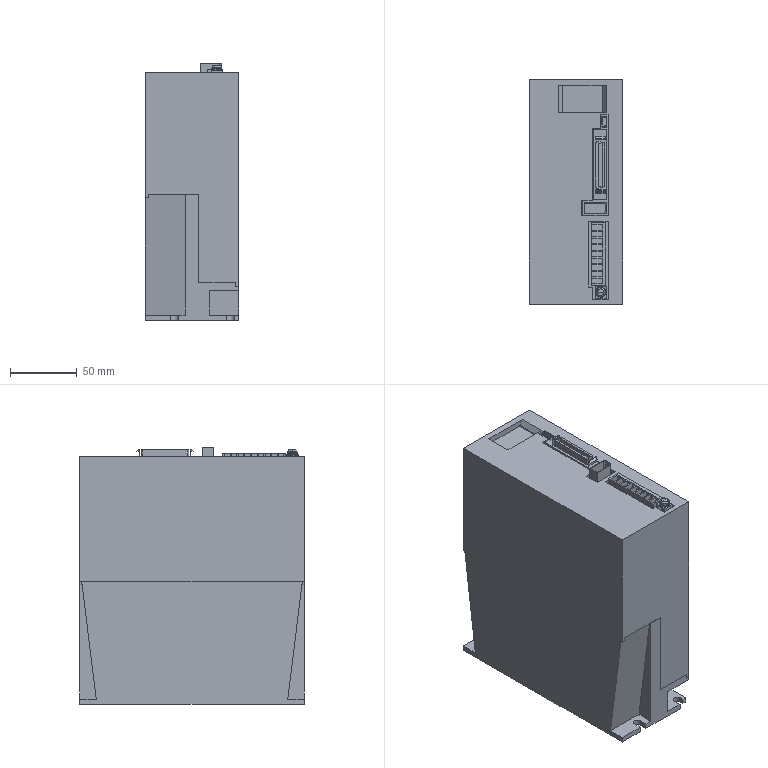Part | STEP file | Servo drive MR-JE-70A | 8 solids | 251 faces | box 70 x 168 x 191.95 mm | volume 896378 mm3 | plane 210 | cylinder 35 | sphere 2 | torus 2 | cone 2 | commonest cylinder face diameters 0.6 x8 1.4 x8 2 x5 4 x4 6 x4 1.2 x2